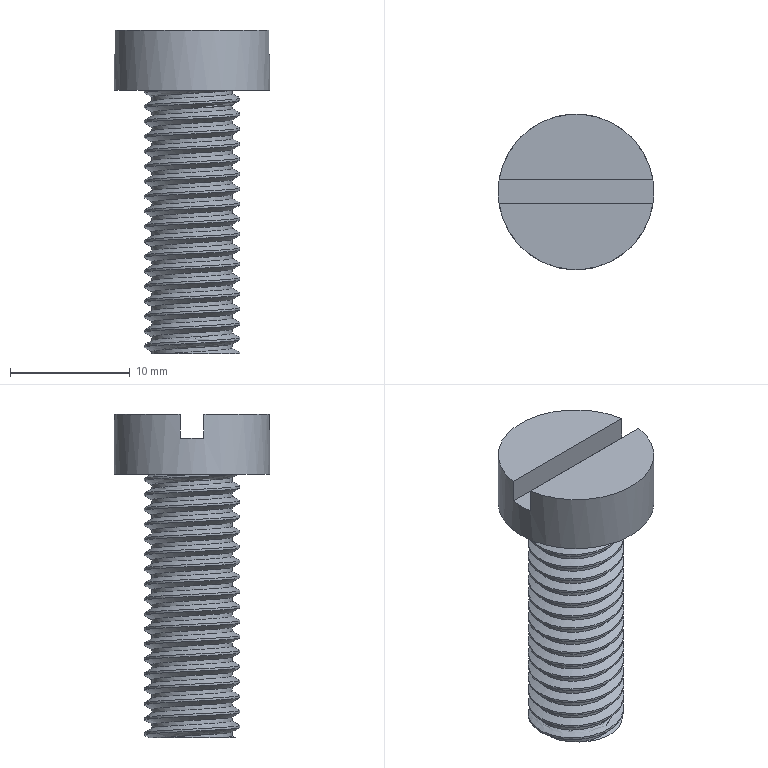Part | NX | features CYLINDER 3, DATUM_CSYS 2, TRIM BODY 2, DATUM_PLANE 1, EXTRUDE 1, SKETCH 1, THREADS 1 | 1 solid | 12 faces | box 13 x 13 x 27 mm | volume 1535 mm3 | plane 7 | cylinder 3 | spline 2 | commonest cylinder face diameters 6.75 x1 8 x1 13 x1